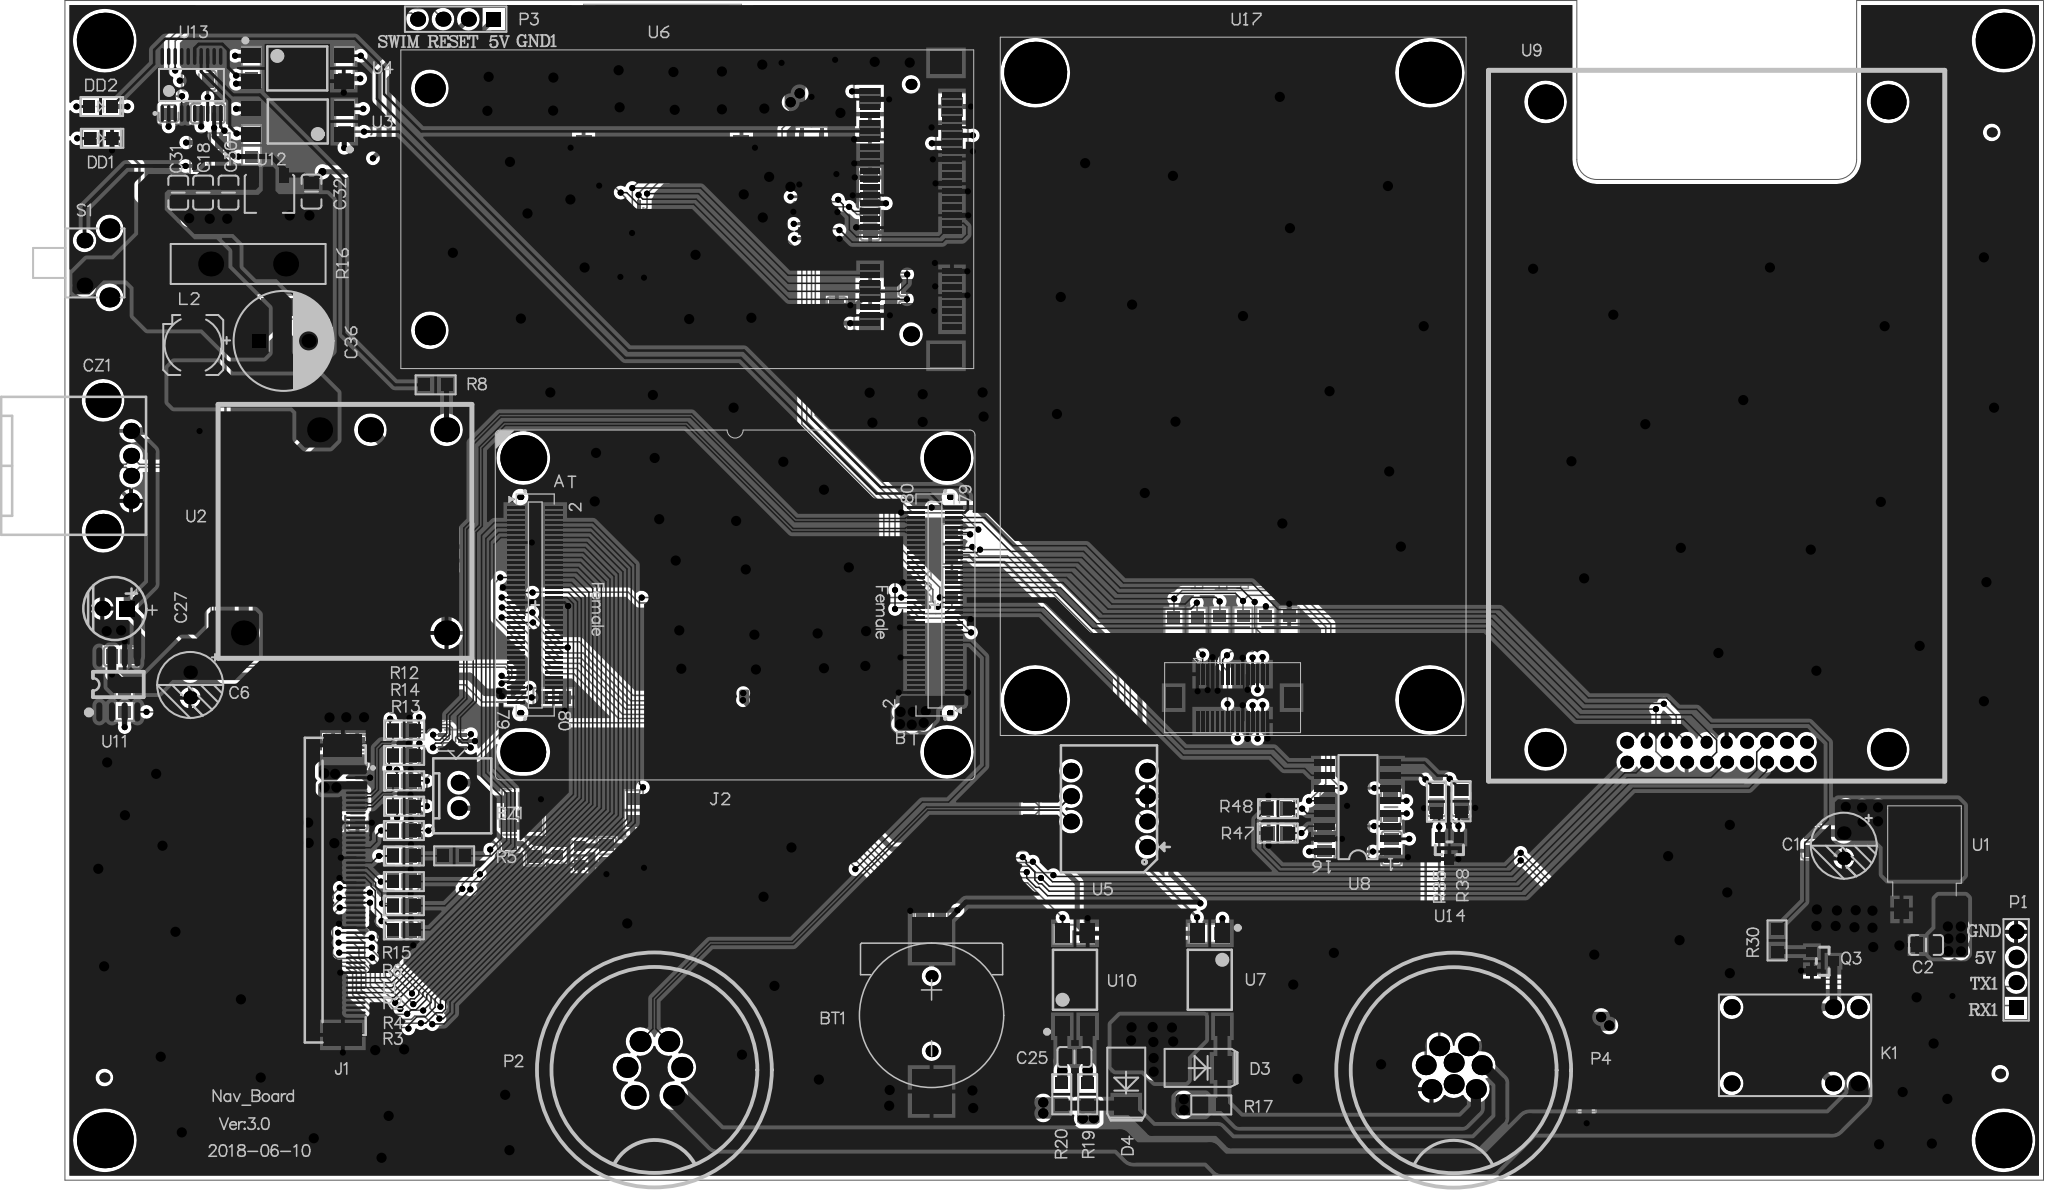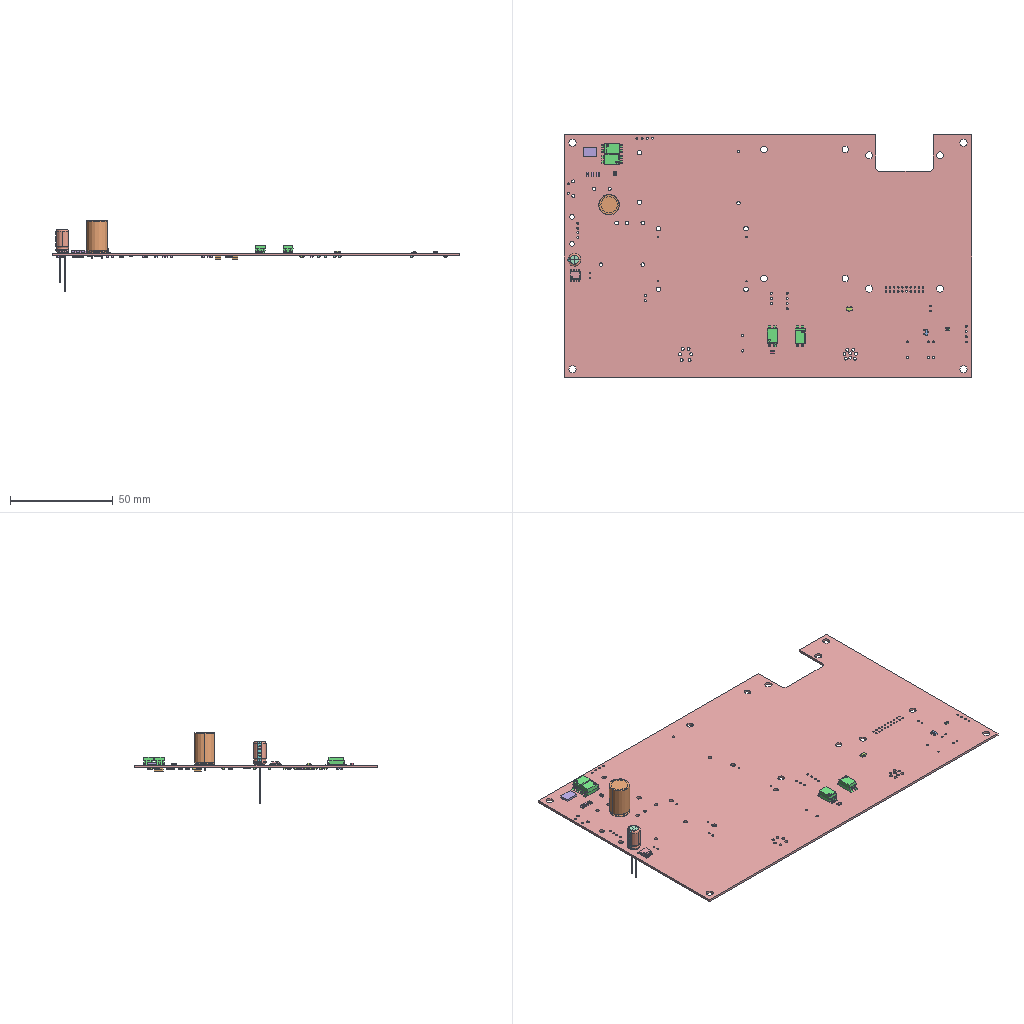Circuit board layout | Altium Designer | box 198 x 118 x 34.2 mm
Layer stack:
# Altium Designer layer stack of  (unit mm; dielectric type: 0 none, 1 core, 2 prepreg, 3 surface material)
index,name,kind,layer,copper_thickness_mm,dielectric_type,dielectric_thickness_mm,dielectric_material,dielectric_constant
0,Top Paste,other,,,,,,
1,Top Overlay,other,,,,,,
2,Top Solder,dielectric,,,3,0.0102,Solder Resist,3.5
3,Top Layer,copper,Top Layer,0.0356,,,,
4,Dielectric1,dielectric,,,1,0.32,FR-4,4.8
5,GND,copper,GND,0.0356,,,,
6,Dielectric5,dielectric,,,2,0.32,FR-4,4.8
7,POWER,copper,POWER,0.0356,,,,
8,Dielectric6,dielectric,,,1,0.32,FR-4,4.8
9,Bottom Layer,copper,Bottom Layer,0.0356,,,,
10,Bottom Solder,dielectric,,,3,0.0102,Solder Resist,3.5
11,Bottom Overlay,other,,,,,,
12,Bottom Paste,other,,,,,,
# drill layer pairs: low layer,high layer
drill_pair,Top Layer,Bottom Layer
Part placement:
Designator,Comment,Layer,Footprint,Center-X(mm),Center-Y(mm),Rotation
R50,10KO,±1%,BottomLayer,0805R,128.6,55.448,90
R49,10KO,±1%,BottomLayer,0805R,126.263,55.448,90
R44,0O,±5%,BottomLayer,0805R,123.977,55.423,270
R43,0O,±5%,BottomLayer,0805R,121.666,55.423,270
R42,0O,±5%,BottomLayer,0805R,119.38,55.397,270
R41,0O,±5%,BottomLayer,0805R,117.069,55.397,270
U23,PESD15VL2BT,BottomLayer,SOT-23,197.206,18.567,180
R48,4.7O,±1%,TopLayer,0805R,127.483,37.313,360
R47,4.7O,±1%,TopLayer,0805R,127.457,34.874,360
P1,2.54 single-row header-4pin,TopLayer,HDR1X4,201.346,21.184,90
C62,15pF,BottomLayer,0805C,127.406,37.338,360
C61,15pF,BottomLayer,0805C,127.432,34.874,360
U21,SN74LVC2T45,BottomLayer,VSSOP-8,81.153,97.765,180
U19,SN74LVC2T45,BottomLayer,VSSOP-8,81.16,95.059,180
U18,RT9193-18GB,BottomLayer,SOT23-5,80.797,106.223,360
U16,PESD3V3L4UG,BottomLayer,SOT-353,62.84,96.698,90
R46,100K,BottomLayer,0805R,82.042,111.1,90
R45,470O,±1%,BottomLayer,0805R,9.652,107.544,180
DD2,RED 0603,TopLayer,LED0805,9.652,107.544,360
C60,22nF,±10%,BottomLayer,0805C,82.093,101.676,90
C59,1µF,±10%,BottomLayer,0805C,79.223,111.023,270
C58,1µF,±10%,BottomLayer,0805C,79.578,101.676,90
C57,10pF,BottomLayer,0805C,83.337,86.766,90
C56,100nF,BottomLayer,0805C,86.665,99.568,90
C55,33pF,BottomLayer,0805C,61.671,92.558,90
C54,33pF,BottomLayer,0805C,64.033,92.558,90
C53,33pF,BottomLayer,0805C,86.665,95.86,270
C52,33pF,BottomLayer,0805C,91.237,91.897,360
C51,33pF,BottomLayer,0805C,91.237,89.56,360
C50,1µF,BottomLayer,0805C,91.237,87.097,360
C49,150µF/6.3V,BottomLayer,CT3528-B,94.844,105.943,90
C48,150µF/6.3V,BottomLayer,CT3528-B,86.665,87.478,90
C47,150µF/6.3V,BottomLayer,CT3528-B,86.639,106.782,270
R37,0O,±5%,BottomLayer,0805R,94.844,59.487,270
R36,0O,±5%,BottomLayer,0805R,94.844,63.779,90
U13,STM8S103F3,TopLayer,TSOP65P640X120-20N,18.745,109.703,90
U12,78L05M,TopLayer,SOT-89,26.492,98.704,180
R34,4.7K  1%,BottomLayer,0805R,20.574,103.937,360
R33,10KO,±1%,BottomLayer,0805R,24.765,103.657,90
P3,2.54 single-row header-4pin,TopLayer,HDR1X4,45.187,116.281,180
C35,100nF,BottomLayer,0805C,20.37,106.853,180
C34,100nF,BottomLayer,0805C,16.459,107.696,90
C33,1uF,BottomLayer,0805C,19.482,110.134,360
C32,100nF,TopLayer,0805C,30.759,99.035,270
C31,100nF,TopLayer,0805C,17.424,98.933,270
C30,100nF,TopLayer,0805C,22.454,98.933,270
C18,100nF,TopLayer,0805C,19.914,98.933,270
BZ1,BUZZER2,TopLayer,XH2.5-2P,45.491,38.633,270
C1,100µF/25V,TopLayer,RB6.3*7,184.099,33.604,270
C2,100nF,TopLayer,0805C,192.329,23.673,180
C3,100nF,BottomLayer,0805C,51.511,38.252,360
C5,100nF,BottomLayer,0805C,180.848,33.985,270
C6,100µF/25V,TopLayer,RB6.3*7,18.618,49.682,270
C7,100nF,BottomLayer,0805C,50.597,34.696,90
C8,15PF,±5%,BottomLayer,0805C,39.827,35.118,360
C9,15PF,±5%,BottomLayer,0805C,39.827,32.588,360
C10,15PF,±5%,BottomLayer,0805C,39.802,27.6,360
C11,15PF,±5%,BottomLayer,0805C,39.802,25.161,360
C12,15PF,±5%,BottomLayer,0805C,39.802,30.089,360
C13,100nF,BottomLayer,0805C,60.274,32.741,90
C14,1nF,CAP,BottomLayer,0805C,39.776,37.556,360
C15,1nF,CAP,BottomLayer,0805C,39.802,42.636,360
C16,1nF,CAP,BottomLayer,0805C,39.802,40.071,360
C17,1nF,CAP,BottomLayer,0805C,39.802,45.176,360
C19,100nF,BottomLayer,0805C,35.357,36.805,90
C20,10µF 10V,BottomLayer,0805C,32.918,36.805,90
C21,10µF 10V,BottomLayer,0805C,35.331,43.002,90
C22,100nF,BottomLayer,0805C,32.918,43.028,270
C24,100nF,BottomLayer,0805C,92.786,27.102,180
C25,1µF,±10%,TopLayer,0805C,107.112,12.471,360
C26,100nF,BottomLayer,0805C,11.684,52.553,180
C27,100µF,25V,TopLayer,CAPPRD250W45D630H800P,11.074,57.328,180
C28,10µF 10V,BottomLayer,0805C,11.455,59.766,180
C29,100nF,BottomLayer,0805C,17.399,75.082,360
D1,1N4148,BottomLayer,SMD-D4148,53.086,34.087,90
D3,P6SMB15A,TopLayer,DO-214,119.634,11.379,360
D4,P6SMB15A,TopLayer,DO-214,112.293,9.906,270
D5,NUP4202W1,BottomLayer,SOT-363,8.865,71.603,360
DD1,RED 0603,TopLayer,LED0805,9.681,104.365,360
H1,Hole,TopLayer,HOLE-3.2,200.076,4.14,0
H2,Hole,TopLayer,HOLE-3.2,200.096,114.127,0
H3,Hole,TopLayer,HOLE-3.2,10.071,114.127,0
H4,Hole,TopLayer,HOLE-3.2,10.084,4.14,0
J1,FPC-50,TopLayer,FFC0.5-50P-A,34.544,29.159,270
L1,1nH,TopLayer,0805R,40.005,32.578,180
P2,6-core,TopLayer,BBD-06PMFP-LC7001,65.075,11.316,180
P4,8-core,TopLayer,BDU-08PMFP-LC7001,145.059,11.401,180
Q1,SS8050LT(1.5A),BottomLayer,SOT-23,56.49,32.639,180
R1,2KO 1%,BottomLayer,0805R,9.808,104.365,360
R2,22O,±5%,TopLayer,0805R,40.005,30.013,180
R3,22O,±5%,TopLayer,0805R,40.005,25.187,180
R4,22O,±5%,TopLayer,0805R,40.005,27.6,180
R5,22O,±5%,TopLayer,0805R,45.034,32.588,180
R6,22O,±5%,TopLayer,0805R,40.005,35.118,180
R8,0O,±5%,TopLayer,0805R,43.18,79.705,180
R9,4.7K  1%,BottomLayer,0805R,62.992,37.16,270
R10,4.7K  1%,BottomLayer,0805R,62.941,32.512,90
R11,1kO,±1%,BottomLayer,0805R,34.087,106.147,90
R12,0O,±5%,TopLayer,0805R,40.03,45.176,180
R13,0O,±5%,TopLayer,0805R,40.03,40.096,180
R14,0O,±5%,TopLayer,0805R,40.03,42.636,180
R15,0O,±5%,TopLayer,0805R,40.03,37.556,180
R17,10kO,±1%,TopLayer,0805R,120.802,7.671,180
R18,2KO 1%,BottomLayer,0805R,120.548,24.841,360
R19,2KO 1%,TopLayer,0805R,108.433,8.738,90
R20,2KO 1%,TopLayer,0805R,105.842,8.738,90
R21,10kO,±1%,BottomLayer,0805R,107.036,24.74,180
R22,10KO,±1%,BottomLayer,0805R,105.842,8.738,270
R23,10KO,±1%,BottomLayer,0805R,108.433,8.738,270
R24,10KO,±1%,BottomLayer,0805R,12.04,48.108,90
R25,22O,±5%,BottomLayer,0805R,17.755,72.72,180
R26,22O,±5%,BottomLayer,0805R,17.78,70.46,180
S1,SW-PB4P,TopLayer,SWICH4.5,9.296,91.897,90
U1,LD1086DT33TR,TopLayer,DPAK,192.176,30.48,360
U2,E2405UHBDD-10W,TopLayer,E2403UHBDD,34.112,65.049,270
U3,PC817,TopLayer,SMD-4,29.388,106.045,180
U20,PESD3V3L4UG,BottomLayer,SOT-353,44.856,44.069,180
U5,CTM1051AM,TopLayer,CTM1051AM,110.566,37.287,90
U7,PC817,TopLayer,SMD-4,120.65,20.193,270
U10,PC817,TopLayer,SMD-4,107.163,20.193,90
U11,SP2526A,TopLayer,SOIC127P600X175-8N,11.43,49.733,90
BT1,BATTERY,TopLayer,BATTERY-1220-1,92.812,16.637,360
CZ1,USB,TopLayer,USB-1400,11.303,71.603,180
D10,1N4148,BottomLayer,SMD-D4148,179.857,13.894,270
Q3,SS8050LT(1.5A),TopLayer,SOT-23,181.991,22.047,360
R27,1KO,±1%,BottomLayer,0805R,54.966,48.438,180
R28,10KO,±1%,BottomLayer,0805R,34.036,111.455,90
R29,2KO 1%,BottomLayer,0805R,24.74,111.506,270
R30,1kO,±1%,TopLayer,0805R,177.419,24.13,270
U4,PC817,TopLayer,SMD-4,29.337,111.354,360
U9,2.0mm dual-row socket-20pin,TopLayer,20PIN-OEM_STARA,171.399,74.981,180
K1,HK4100F-DC5V-SHG 0.2W,TopLayer,HK4100F,179.222,13.64,180
R31,10KO,±1%,BottomLayer,0805R,20.599,101.6,360
R32,120O 1%,BottomLayer,0805R,102.616,37.313,90
C38,100nF,BottomLayer,0805C,135.611,34.265,270
C39,100nF,BottomLayer,0805C,132.156,33.934,90
C40,100nF,BottomLayer,0805C,138.836,33.35,270
C41,100nF,BottomLayer,0805C,138.786,37.465,270
C42,100nF,BottomLayer,0805C,135.611,38.481,270
C43,15pF,BottomLayer,0805C,145.796,38.278,270
C44,15pF,BottomLayer,0805C,143.332,38.252,270
L2,4.7uH,TopLayer,SLF6045,18.926,83.69,270
R16,14D560K,TopLayer,14D560K,24.419,91.796,90
R35,4.7O,±1%,TopLayer,0805R,143.332,38.024,90
R38,4.7O,±1%,TopLayer,0805R,145.796,38.049,90
R39,0O,±1%,BottomLayer,0805R,158.369,9.017,270
R40,0O,±1%,BottomLayer,0805R,158.394,14.656,90
U8,SP3232EEN,TopLayer,SOP16-6.6,135.484,37.465,180
U14,PESD15VL2BT,TopLayer,SOT-23,144.628,33.35,270
U17,HX-DU1006D,TopLayer,HX-DU1006D,122.936,78.492,180
U15,USIM,BottomLayer,SIM,65.888,108.433,0
U6,ME909s-821,TopLayer,PCIE_0,68.729,97.26,90
J2,HEADER 40X2,TopLayer,AM3352B,73.152,57.683,360
C4,1nF/2kV,BottomLayer,C1206,23.978,63.475,270
C23,4.7uF/25V,BottomLayer,C1206,27.94,87.478,180
C36,330µF/35V,TopLayer,CAPPR5.0-10X16-0.8,27.965,84.099,360
C37,1nF/2kV,BottomLayer,C1206,44.272,63.525,270
Pad and via stacks:
# Altium Designer via and pad stacks of  (unit mm). Each distinct definition once, with the count of objects using it.
# via: kind,start_layer,end_layer,hole_mm,diameter_mm,mode(0 simple;1 top-mid-bottom;2 full stack),diameter_per_layer,count,example_net
# pad: kind,layer,hole_mm,hole_type(0 round;1 square;2 slot),plating,top_size,top_shape(1 round;2 rect;3 octagon;9 rounded rect),mid_size,bottom_size,mode,footprint,size_per_layer,count,example
pad,Top Layer,0,0,unplated,1.45x1.15,2,1.45x1.15,1.45x1.15,0,0805C,,12,C2.1
pad,Top Layer,0,0,plated,1.5x2,2,1.5x2,1.5x2,0,DPAK,,2,U1.3
pad,Top Layer,0,0,plated,7x7,2,7x7,7x7,0,DPAK,,1,U1.2
pad,Top Layer,0,0,plated,2.1x0.3,2,2.1x0.3,2.1x0.3,0,HX-DU1006D,,30,U17.29
pad,Top Layer,0,0,plated,2.1x1.6,2,2.1x1.6,2.1x1.6,0,HX-DU1006D,,2,U17.31
pad,Top Layer,0,0,plated,1.8x0.3,2,1.8x0.3,1.8x0.3,0,AM3352B,,160,J2.A65
pad,Top Layer,0,0,plated,0.6x2,2,0.6x2,0.6x2,0,PCIE_0,,52,U6.52
pad,Top Layer,0,0,plated,2.3x3.2,2,2.3x3.2,2.3x3.2,0,PCIE_0,,2,U6.54
pad,Top Layer,0,0,plated,0.6096x2.032,2,0.6096x2.032,0.6096x2.032,0,SOP16-6.6,,16,U8.14
pad,Top Layer,0,0,plated,4.5x4,2,4.5x4,4.5x4,0,BATTERY-1220-1,,2,BT1.1
pad,Top Layer,0,0,plated,1.932x0.6096,1,1.932x0.6096,1.932x0.6096,0,SOIC127P600X175-8N,,8,U11.1
pad,Top Layer,0,0,plated,1.5x2,2,1.5x2,1.5x2,0,SMD-4,,16,U3.1
pad,Top Layer,0,0,plated,0.25x2,1,0.25x2,0.25x2,0,FFC0.5-50P-A,,49,J1.50
pad,Top Layer,0,0,plated,0.25x2,2,0.25x2,0.25x2,0,FFC0.5-50P-A,,1,J1.1
pad,Top Layer,0,0,plated,2.286x3.81,2,2.286x3.81,2.286x3.81,0,FFC0.5-50P-A,,2,J1.52
pad,Top Layer,0,0,plated,2.4x1.8,2,2.4x1.8,2.4x1.8,0,DO-214,,4,D3.2
pad,Top Layer,0,0,plated,0.9906x1.499,2,0.9906x1.499,0.9906x1.499,0,SOT-89,,3,U12.3
pad,Top Layer,0,0,plated,2.007x2.007,2,2.007x2.007,2.007x2.007,0,SOT-89,,1,U12.2
pad,Top Layer,0,0,plated,0.35x1.7,1,0.35x1.7,0.35x1.7,0,TSOP65P640X120-20N,,20,U13.11
pad,Top Layer,0,0,plated,1.2x1.3,2,1.2x1.3,1.2x1.3,0,LED0805,,4,DD2.2
pad,Top Layer,0,0,plated,1.2x1.3,2,1.2x1.3,1.2x1.3,0,0805R,,38,R48.2
pad,Top Layer,0,0,plated,1x1,1,1x1,1x1,0,,,3,0
pad,Top Layer,0,0,plated,0.9144x1.016,2,0.9144x1.016,0.9144x1.016,0,SOT-23,,6,U14.3
pad,Top Layer,0,0,plated,1.5x2.2,2,1.5x2.2,1.5x2.2,0,SLF6045,,2,L2.1
pad,Multi-Layer,3.2,0,plated,6.2x6.2,1,6.2x6.2,6.2x6.2,0,HX-DU1006D,,4,U17.0
pad,Multi-Layer,0.6,0,unplated,0.6x0.6,1,0.6x0.6,0.6x0.6,0,AM3352B,,8,J2.0
pad,Multi-Layer,2.2,0,plated,4.6x4.6,1,4.6x4.6,4.6x4.6,0,AM3352B,,3,J2.4
pad,Multi-Layer,2.2,0,plated,4x4.6,1,4x4.6,4x4.6,0,AM3352B,,1,J2.2
pad,Multi-Layer,1.6,0,unplated,1.6x1.6,1,1.6x1.6,1.6x1.6,0,PCIE_0,,1,U6.0
pad,Multi-Layer,1.1,0,unplated,1.1x1.1,1,1.1x1.1,1.1x1.1,0,PCIE_0,,1,U6.0
pad,Multi-Layer,2.2,0,unplated,3x3,1,3x3,3x3,0,PCIE_0,,2,U6.0
pad,Multi-Layer,1.6,0,plated,2.5x2.5,1,2.5x2.5,2.5x2.5,0,14D560K,,2,R16.2
pad,Multi-Layer,0.9,0,plated,1.6x1.6,1,1.6x1.6,1.6x1.6,0,HK4100F,,6,K1.1
pad,Multi-Layer,0.7366,0,plated,1.3x1.3,1,1.3x1.3,1.3x1.3,0,20PIN-OEM_STARA,,15,U9.2
pad,Multi-Layer,0.7366,0,plated,1.2x1.3,1,1.2x1.3,1.2x1.3,0,20PIN-OEM_STARA,,5,U9.10
pad,Multi-Layer,3.5,0,plated,3.5x3.5,1,3.5x3.5,3.5x3.5,0,20PIN-OEM_STARA,,4,U9.21
pad,Multi-Layer,1,0,plated,1.6x1.6,1,1.6x1.6,1.6x1.6,0,USB-1400,,4,CZ1.3
pad,Multi-Layer,2.3,0,plated,3.5x3.5,1,3.5x3.5,3.5x3.5,0,USB-1400,,2,CZ1.6
pad,Multi-Layer,1.2,0,plated,1.2x1.2,1,1.2x1.2,1.2x1.2,0,BATTERY-1220-1,,2,BT1.0
pad,Multi-Layer,1,0,plated,1.6x1.6,1,1.6x1.6,1.6x1.6,0,CTM1051AM,,7,U5.1
pad,Multi-Layer,1,0,plated,1.575x1.575,1,1.575x1.575,1.575x1.575,0,SWICH4.5,,2,S1.1
pad,Multi-Layer,1.5,0,plated,2x2,1,2x2,2x2,0,SWICH4.5,,2,S1.4
pad,Multi-Layer,1.4,0,plated,2x2,1,2x2,2x2,0,BDU-08PMFP-LC7001,,8,P4.6
pad,Multi-Layer,1.4,0,plated,2.1x2.1,1,2.1x2.1,2.1x2.1,0,BBD-06PMFP-LC7001,,6,P2.6
pad,Multi-Layer,3.5,0,plated,5.6x5.6,1,5.6x5.6,5.6x5.6,0,HOLE-3.2,,4,H1.8
pad,Multi-Layer,0.8,0,plated,1.524x1.524,2,1.524x1.524,1.524x1.524,0,CAPPRD250W45D630H800P,,1,C27.1
pad,Multi-Layer,0.8,0,plated,1.524x1.524,1,1.524x1.524,1.524x1.524,0,CAPPRD250W45D630H800P,,1,C27.2
pad,Multi-Layer,1,0,plated,1.6x1.6,1,1.6x1.6,1.6x1.6,0,XH2.5-2P,,2,BZ1.2
pad,Multi-Layer,0.9,0,plated,1.5x1.5,1,1.5x1.5,1.5x1.5,0,HDR1X4,,6,P1.4
pad,Multi-Layer,0.9,0,plated,1.5x1.5,2,1.5x1.5,1.5x1.5,0,HDR1X4,,2,P1.1
pad,Multi-Layer,1.8,0,plated,2.5x2.5,1,2.5x2.5,2.5x2.5,0,E2403UHBDD,,5,U2.1
pad,Multi-Layer,0.75,0,plated,1.35x1.35,1,1.35x1.35,1.35x1.35,0,RB6.3*7,,4,C6.2
pad,Multi-Layer,0.8,0,plated,1.4x1.4,1,1.4x1.4,1.4x1.4,0,CAPPR5.0-10X16-0.8,,1,C36.2
pad,Multi-Layer,0.8,0,plated,1.4x1.4,2,1.4x1.4,1.4x1.4,0,CAPPR5.0-10X16-0.8,,1,C36.1
pad,Bottom Layer,0,0,plated,0.35x0.896,2,0.35x0.896,0.35x0.896,0,SOT-353,,10,U20.4
pad,Bottom Layer,0,0,plated,1.2x1.3,2,1.2x1.3,1.2x1.3,0,0805R,,60,R9.1
pad,Bottom Layer,0,0,unplated,1.45x1.15,2,1.45x1.15,1.45x1.15,0,0805C,,88,C3.1
pad,Bottom Layer,0,0,plated,0.9144x1.016,2,0.9144x1.016,0.9144x1.016,0,SOT-23,,6,Q1.3
pad,Bottom Layer,0,0,plated,1.27x1.5,2,1.27x1.5,1.27x1.5,0,SMD-D4148,,4,D1.2
pad,Bottom Layer,0,0,plated,0.35x0.896,2,0.35x0.896,0.35x0.896,0,SOT-363,,6,D5.5
pad,Bottom Layer,0,0,plated,2x2.2,2,2x2.2,2x2.2,0,CT3528-B,,6,C49.2
pad,Bottom Layer,0,0,plated,0.4x1,2,0.4x1,0.4x1,0,SOT23-5,,5,U18.1
pad,Bottom Layer,0,0,plated,0.3x0.8,2,0.3x0.8,0.3x0.8,0,VSSOP-8,,16,U21.8
pad,Bottom Layer,0,0,plated,1x1,1,1x1,1x1,0,,,3,0
pad,Bottom Layer,0,0,plated,0.65x1.35,2,0.65x1.35,0.65x1.35,0,SIM,,6,U15.3
pad,Bottom Layer,0,0,plated,1.55x2.6,2,1.55x2.6,1.55x2.6,0,SIM,,4,U15.9
pad,Bottom Layer,0,0,plated,1.6x1.8,2,1.6x1.8,1.6x1.8,0,C1206,,6,C37.1
via,Top Layer,Bottom Layer,0.3048,0.6096,0,,258,232TX1
via,Top Layer,Bottom Layer,0.381,0.762,0,,1,5V
via,Top Layer,Bottom Layer,0.508,1.016,0,,197,NetC25_1
Copper pours:
name,layer,net,type(0 solid;1 hatched;2 none)
Top Layer-No Net,Bottom Layer,USB0_VBUS_5V,0
Top Layer-No Net,Bottom Layer,VDD_12V,0
Top Layer-No Net,Bottom Layer,VDD_5V,0
Top Layer-No Net,Bottom Layer,VDD_3.3,0
Top Layer-No Net,Bottom Layer,VDD_3.3,0
Top Layer-No Net,Bottom Layer,VDD_3.3,0
Top Layer-No Net,Bottom Layer,GND1,0
Top Layer-No Net,Bottom Layer,GND1,0
Top Layer-No Net,Bottom Layer,GND,0
Top Layer-No Net,Top Layer,GND1,0
Top Layer-No Net,Top Layer,VDD_12V,0
Top Layer-No Net,Top Layer,USB0_VBUS_5V,0
Top Layer-No Net,Top Layer,NetC4_1,0
Top Layer-No Net,Top Layer,VDD_5V,0
Top Layer-No Net,Top Layer,VDD_12V,0
Top Layer-No Net,Top Layer,VDD_5V,0
Top Layer-No Net,Top Layer,VDD_5V,0
Top Layer-No Net,Top Layer,VDD_3.3,0
Top Layer-No Net,Top Layer,VDD_5V,0
Top Layer-No Net,Top Layer,VDD_3.3,0
Top Layer-No Net,Top Layer,GND1,0
Top Layer-No Net,Top Layer,GND,0
Design rules, without the lines most boards share:
# Altium Designer design rules of  (exported by Altium Designer, unit mm)
# columns: name | kind | enabled | priority | scope1 | scope2 | descriptor | typed fields (field=value)
PolygonConnect_2 | 20 | enabled | 1 | All | isvia | Polygon Connect Rule(Direct Connect )(Conductor Width=10mil) (Relief Angle=90 Angle) (Entries=4) (Air Gap Width=10mil) (All),(isvia) | connect_style(0=relief,1=direct,2=none)=1 relief_conductor_width=0.254 relief_entries=4
PolygonConnect_1 | 20 | enabled | 2 | InNet(GND) | All | Polygon Connect Rule(Relief Connect )(Conductor Width=15mil) (Relief Angle=90 Angle) (Entries=4) (Air Gap Width=10mil) (InNet(GND)),(All) | connect_style(0=relief,1=direct,2=none)=0 relief_conductor_width=0.381 relief_entries=4
Clearance_1 | 0 | enabled | 1 | InPolygon | All | Clearance Constraint (Gap=6mil) (InPolygon),(All) | gap=0.1524
SilkToSilkClearance | 55 | disabled | 1 | All | All | Silk to Silk (Clearance=10mil) (Disabled)(All),(All) |
SilkscreenOverComponentPads | 54 | disabled | 1 | IsPad | All | Silk To Solder Mask (Clearance=10mil) (Disabled)(IsPad),(All) |
MinimumSolderMaskSliver | 53 | disabled | 1 | All | All | Minimum Solder Mask Sliver (Gap=10mil) (Disabled)(All),(All) |
HoleToHoleClearance | 52 | enabled | 1 | All | All | Hole To Hole Clearance (Gap=0mil) (All),(All) | gap=0
DiffPairsRouting | 51 | enabled | 1 | All | All | Differential Pairs Uncoupled Length using the Gap Constraints (Min=6mil) (Max=6mil) (Prefered=6mil)  and Width Constraints (Min=15mil) (Max=15mil) (Prefered=15mil) (All) |
HoleSize | 42 | enabled | 1 | All | All | Hole Size Constraint (Min=1mil) (Max=10000mil) (All) |
Height | 50 | enabled | 1 | All | All | Height Constraint (Min=0mil) (Max=70503.27mil) (Prefered=500mil) (All) | min_height=0 max_height=1790.783
ComponentClearance | 24 | disabled | 1 | All | All | Component Clearance Constraint ( Horizontal Gap = 10mil, Vertical Gap = 10mil ) (Disabled)(All),(All)  | gap=0.254
SolderMaskExpansion | 13 | enabled | 1 | All | All | Solder Mask Expansion (Expansion =4mil) (All) | expansion=0.1016
PasteMaskExpansion | 14 | enabled | 1 | All | All | Paste Mask Expansion (Expansion =0mil) (All) | expansion=0
RoutingVias | 11 | enabled | 1 | All | All | Routing Via (MinHoleWidth=12mil) (MaxHoleWidth=12mil) (PreferredHoleWidth=12mil) (MinWidth=24mil) (MaxWidth=24mil) (PreferedWidth=24mil) (All) | via_min_hole=0.3048 via_max_hole=0.3048 via_preferred_diameter=0.6096 via_preferred_hole=0.3048
Width | 2 | enabled | 1 | All | All | Width Constraint (Min=6mil) (Max=80mil) (Preferred=6mil) (All) |
PolygonConnect | 20 | enabled | 3 | All | All | Polygon Connect Rule(Direct Connect )(Conductor Width=10mil) (Relief Angle=90 Angle) (Entries=4) (Air Gap Width=10mil) (All),(All) | connect_style(0=relief,1=direct,2=none)=1 relief_conductor_width=0.254 relief_entries=4
PlaneConnect | 6 | enabled | 1 | All | All | Power Plane Connect Rule(Direct Connect )(Expansion=20mil) (Conductor Width=10mil) (Air Gap=10mil) (Entries=4) (All) | relief_conductor_width=0.254 relief_entries=4 relief_expansion=0.508
Clearance | 0 | enabled | 2 | All | All | Clearance Constraint (Gap=6mil) (All),(All) | gap=0.1524
Classes set for this board:
# Altium Designer classes of  (member kind: 0 net, 1 component, 2 from-to, 3 pad, 4 layer, 5 differential pair, 6 design channel, 7 polygon, 8 structure, 9 xSignal)
# columns: class name | member kind | superclass | members
Nav_Board-V3.0 | 1 | no | BZ1; C1; C2; C3; C4; C5; C6; C7; C8; C9; C10; C11; C12; C13; C14; C15; C16; C17; C19; C20; C21; C22; C24; C25; C26; C27; C28; C29; D1; DD1; H1; H2; H3; H4; J1; L1; P2; P4; R1; R2; R3; R4; R5; R6; R8; R9; R10; R11; R12; R13; R14; R15; R17; R18; R19; R20; R21; R22; R23; R24; R25; R26; S1; U1; U2; U3; U5; U7; BT1; BZ1; C1; C2; C3; C4; C5; C6; C7; C8; C9; C10; C11; C12; C13; C14; C15; C16; C17; C19; C20; C21; C22; C24; C25; C26; C27; C28; C29; CZ1; D1; D3; D4; D5; DD1; H1; H2; H3; H4; J1; J3; L1; P2; P4; Q1; R1; R2; R3; R4; R5; R6; R8; R9; R10; R11; R12; R13; R14; R15; R17; R18; R19; R20; R21; R22; R23; R24; R25; R26; S1; U1; U2; U3; U5; U7; U9; U10; U11; CZ1; J2; Q3; R27; R28; R29; R30; U20; D5; U20; D10; D10; U20; K1; U4; R31; R32; C18; C30; C31; C32; C33; C34; C35; P3; R33; R34; U12; U13; R36; R37; C23; C36; C37; C38; C39; C40; C41; C42; C43; C44; L2; R16; R35; R38; R39; R40; U8; U14; C47; C48; C49; C50; C51; C52; C53; C54; C55; C56; C57; C58; C59; C60; DD2; R45; R46; U16; U18; U17; U19; U21; U15; U15; U6; J2; C61; C62; P1; R47; R48; U23; R41; R42; R43; R44; R49; R50; C4; C23; C36; C37;